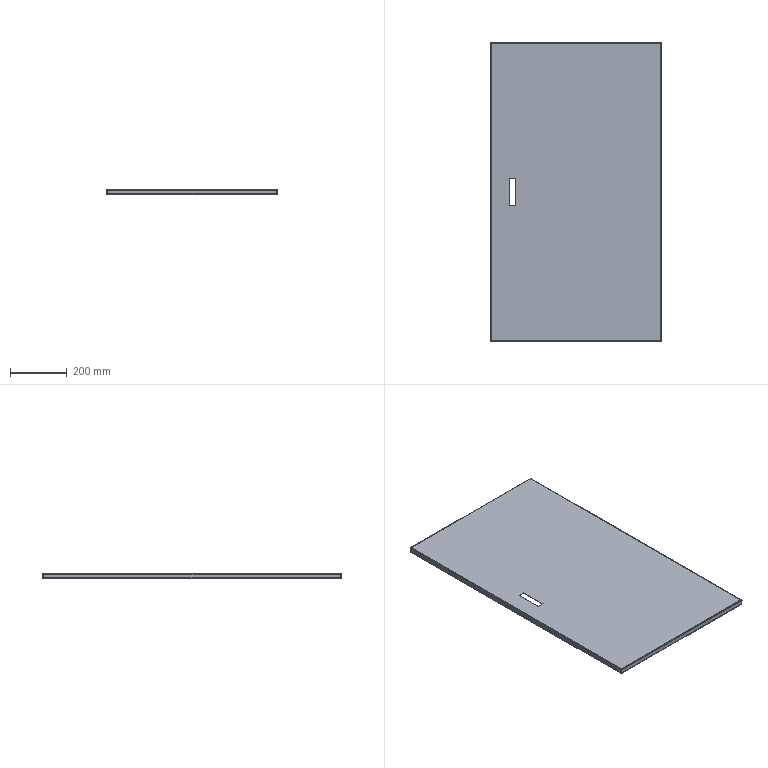Part | SolidWorks | features EdgeFlange 2, CornerFeat 1, FlatPattern 1, ICE 1, SMBaseFlange 1, SheetMetal 1 | 1 solid | 74 faces | box 600 x 1050 x 20 mm | volume 1074617 mm3 | plane 42 | spline 16 | cylinder 16 | commonest cylinder face diameters 3 x8 6 x8